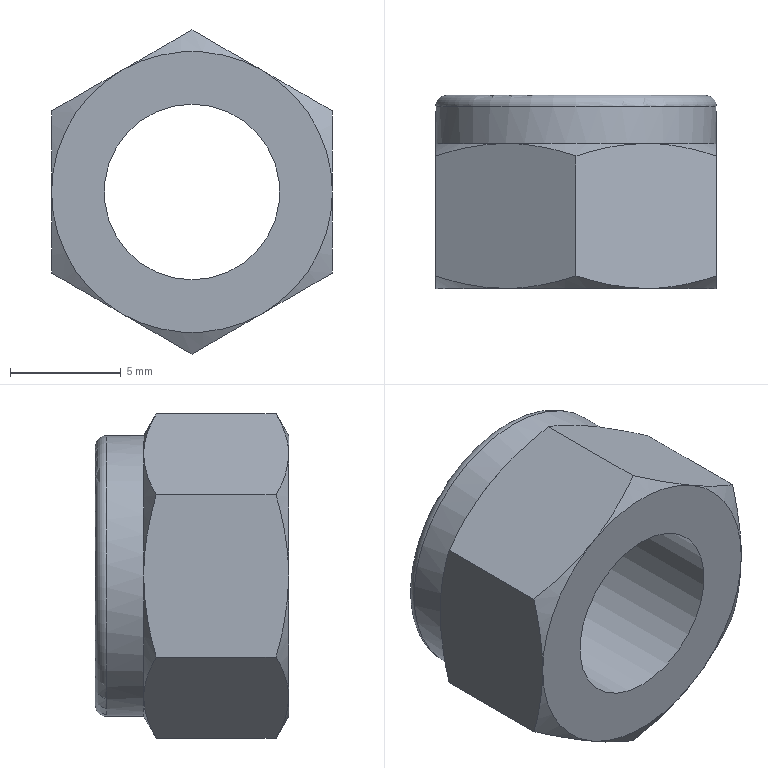Part | NX | features solid 2 | 1 solid | 23 faces | box 12.7 x 8.738 x 14.665 mm | volume 753.009 mm3 | cone 12 | plane 8 | cylinder 2 | torus 1 | commonest cylinder face diameters 7.938 x1 12.7 x1
STEP:
#1=CARTESIAN_POINT('',(0.,5.986,7.332));
#2=VERTEX_POINT('',#1);
#3=CARTESIAN_POINT('',(3.175,6.553,5.499));
#4=VERTEX_POINT('',#3);
#5=CARTESIAN_POINT('',(0.,5.986,7.332));
#6=CARTESIAN_POINT('',(1.039,6.332,6.733));
#7=CARTESIAN_POINT('',(2.093,6.553,6.124));
#8=CARTESIAN_POINT('',(3.175,6.553,5.499));
#9=B_SPLINE_CURVE_WITH_KNOTS('',3,(#5,#6,#7,#8),.UNSPECIFIED.,.F.,.F.,(4,4),(0.000000238,0.00371),.UNSPECIFIED.);
#10=EDGE_CURVE('',#2,#4,#9,.T.);
#11=ORIENTED_EDGE('',*,*,#10,.T.);
#12=CARTESIAN_POINT('',(-3.175,6.553,5.499));
#13=VERTEX_POINT('',#12);
#14=CARTESIAN_POINT('',(0.,6.553,0.));
#15=DIRECTION('',(0.,-1.,0.));
#16=DIRECTION('',(0.,0.,-1.));
#17=AXIS2_PLACEMENT_3D('',#14,#15,#16);
#18=CIRCLE('',#17,6.35);
#19=EDGE_CURVE('',#4,#13,#18,.T.);
#20=ORIENTED_EDGE('',*,*,#19,.T.);
#21=CARTESIAN_POINT('',(-3.175,6.553,5.499));
#22=CARTESIAN_POINT('',(-2.097,6.553,6.122));
#23=CARTESIAN_POINT('',(-1.036,6.331,6.734));
#24=CARTESIAN_POINT('',(0.,5.986,7.332));
#25=B_SPLINE_CURVE_WITH_KNOTS('',3,(#21,#22,#23,#24),.UNSPECIFIED.,.F.,.F.,(4,4),(0.00371,0.007406),.UNSPECIFIED.);
#26=EDGE_CURVE('',#13,#2,#25,.T.);
#27=ORIENTED_EDGE('',*,*,#26,.T.);
#28=EDGE_LOOP('',(#11,#20,#27));
#29=FACE_BOUND('',#28,.T.);
#30=CARTESIAN_POINT('',(0.,6.553,0.));
#31=DIRECTION('',(0.,-1.,0.));
#32=DIRECTION('',(0.,0.,-1.));
#33=AXIS2_PLACEMENT_3D('',#30,#31,#32);
#34=CONICAL_SURFACE('',#33,6.35,1.047);
#35=ADVANCED_FACE('',(#29),#34,.T.);
#36=CARTESIAN_POINT('',(-6.35,5.986,3.666));
#37=VERTEX_POINT('',#36);
#38=CARTESIAN_POINT('',(-6.35,5.986,3.666));
#39=CARTESIAN_POINT('',(-5.311,6.332,4.266));
#40=CARTESIAN_POINT('',(-4.257,6.553,4.875));
#41=CARTESIAN_POINT('',(-3.175,6.553,5.499));
#42=B_SPLINE_CURVE_WITH_KNOTS('',3,(#38,#39,#40,#41),.UNSPECIFIED.,.F.,.F.,(4,4),(0.000000238,0.00371),.UNSPECIFIED.);
#43=EDGE_CURVE('',#37,#13,#42,.T.);
#44=ORIENTED_EDGE('',*,*,#43,.T.);
#45=CARTESIAN_POINT('',(-6.35,6.553,0.));
#46=VERTEX_POINT('',#45);
#47=CARTESIAN_POINT('',(0.,6.553,0.));
#48=DIRECTION('',(0.,-1.,0.));
#49=DIRECTION('',(0.,0.,-1.));
#50=AXIS2_PLACEMENT_3D('',#47,#48,#49);
#51=CIRCLE('',#50,6.35);
#52=EDGE_CURVE('',#13,#46,#51,.T.);
#53=ORIENTED_EDGE('',*,*,#52,.T.);
#54=CARTESIAN_POINT('',(-6.35,6.553,0.));
#55=CARTESIAN_POINT('',(-6.35,6.553,1.241));
#56=CARTESIAN_POINT('',(-6.35,6.328,2.48));
#57=CARTESIAN_POINT('',(-6.35,5.986,3.666));
#58=B_SPLINE_CURVE_WITH_KNOTS('',3,(#54,#55,#56,#57),.UNSPECIFIED.,.F.,.F.,(4,4),(0.01042,0.01413),.UNSPECIFIED.);
#59=EDGE_CURVE('',#46,#37,#58,.T.);
#60=ORIENTED_EDGE('',*,*,#59,.T.);
#61=EDGE_LOOP('',(#44,#53,#60));
#62=FACE_BOUND('',#61,.T.);
#63=CARTESIAN_POINT('',(0.,6.553,0.));
#64=DIRECTION('',(0.,-1.,0.));
#65=DIRECTION('',(0.,0.,-1.));
#66=AXIS2_PLACEMENT_3D('',#63,#64,#65);
#67=CONICAL_SURFACE('',#66,6.35,1.047);
#68=ADVANCED_FACE('',(#62),#67,.T.);
#69=CARTESIAN_POINT('',(-6.35,5.986,-3.666));
#70=VERTEX_POINT('',#69);
#71=CARTESIAN_POINT('',(-6.35,5.986,-3.666));
#72=CARTESIAN_POINT('',(-6.35,6.331,-2.473));
#73=CARTESIAN_POINT('',(-6.35,6.553,-1.24));
#74=CARTESIAN_POINT('',(-6.35,6.553,0.));
#75=B_SPLINE_CURVE_WITH_KNOTS('',3,(#71,#72,#73,#74),.UNSPECIFIED.,.F.,.F.,(4,4),(0.006707,0.01042),.UNSPECIFIED.);
#76=EDGE_CURVE('',#70,#46,#75,.T.);
#77=ORIENTED_EDGE('',*,*,#76,.T.);
#78=CARTESIAN_POINT('',(-3.175,6.553,-5.499));
#79=VERTEX_POINT('',#78);
#80=CARTESIAN_POINT('',(0.,6.553,0.));
#81=DIRECTION('',(0.,-1.,0.));
#82=DIRECTION('',(0.,0.,-1.));
#83=AXIS2_PLACEMENT_3D('',#80,#81,#82);
#84=CIRCLE('',#83,6.35);
#85=EDGE_CURVE('',#46,#79,#84,.T.);
#86=ORIENTED_EDGE('',*,*,#85,.T.);
#87=CARTESIAN_POINT('',(-3.175,6.553,-5.499));
#88=CARTESIAN_POINT('',(-4.253,6.553,-4.877));
#89=CARTESIAN_POINT('',(-5.314,6.331,-4.264));
#90=CARTESIAN_POINT('',(-6.35,5.986,-3.666));
#91=B_SPLINE_CURVE_WITH_KNOTS('',3,(#87,#88,#89,#90),.UNSPECIFIED.,.F.,.F.,(4,4),(0.00371,0.007406),.UNSPECIFIED.);
#92=EDGE_CURVE('',#79,#70,#91,.T.);
#93=ORIENTED_EDGE('',*,*,#92,.T.);
#94=EDGE_LOOP('',(#77,#86,#93));
#95=FACE_BOUND('',#94,.T.);
#96=CARTESIAN_POINT('',(0.,6.553,0.));
#97=DIRECTION('',(0.,-1.,0.));
#98=DIRECTION('',(0.,0.,-1.));
#99=AXIS2_PLACEMENT_3D('',#96,#97,#98);
#100=CONICAL_SURFACE('',#99,6.35,1.047);
#101=ADVANCED_FACE('',(#95),#100,.T.);
#102=CARTESIAN_POINT('',(0.,5.986,-7.332));
#103=VERTEX_POINT('',#102);
#104=CARTESIAN_POINT('',(0.,5.986,-7.332));
#105=CARTESIAN_POINT('',(-1.039,6.332,-6.733));
#106=CARTESIAN_POINT('',(-2.093,6.553,-6.124));
#107=CARTESIAN_POINT('',(-3.175,6.553,-5.499));
#108=B_SPLINE_CURVE_WITH_KNOTS('',3,(#104,#105,#106,#107),.UNSPECIFIED.,.F.,.F.,(4,4),(0.000000238,0.00371),.UNSPECIFIED.);
#109=EDGE_CURVE('',#103,#79,#108,.T.);
#110=ORIENTED_EDGE('',*,*,#109,.T.);
#111=CARTESIAN_POINT('',(3.175,6.553,-5.499));
#112=VERTEX_POINT('',#111);
#113=CARTESIAN_POINT('',(0.,6.553,0.));
#114=DIRECTION('',(0.,-1.,0.));
#115=DIRECTION('',(0.,0.,-1.));
#116=AXIS2_PLACEMENT_3D('',#113,#114,#115);
#117=CIRCLE('',#116,6.35);
#118=EDGE_CURVE('',#79,#112,#117,.T.);
#119=ORIENTED_EDGE('',*,*,#118,.T.);
#120=CARTESIAN_POINT('',(3.175,6.553,-5.499));
#121=CARTESIAN_POINT('',(2.097,6.553,-6.122));
#122=CARTESIAN_POINT('',(1.036,6.331,-6.734));
#123=CARTESIAN_POINT('',(0.,5.986,-7.332));
#124=B_SPLINE_CURVE_WITH_KNOTS('',3,(#120,#121,#122,#123),.UNSPECIFIED.,.F.,.F.,(4,4),(0.00371,0.007406),.UNSPECIFIED.);
#125=EDGE_CURVE('',#112,#103,#124,.T.);
#126=ORIENTED_EDGE('',*,*,#125,.T.);
#127=EDGE_LOOP('',(#110,#119,#126));
#128=FACE_BOUND('',#127,.T.);
#129=CARTESIAN_POINT('',(0.,6.553,0.));
#130=DIRECTION('',(0.,-1.,0.));
#131=DIRECTION('',(0.,0.,-1.));
#132=AXIS2_PLACEMENT_3D('',#129,#130,#131);
#133=CONICAL_SURFACE('',#132,6.35,1.047);
#134=ADVANCED_FACE('',(#128),#133,.T.);
#135=CARTESIAN_POINT('',(6.35,5.986,-3.666));
#136=VERTEX_POINT('',#135);
#137=CARTESIAN_POINT('',(6.35,5.986,-3.666));
#138=CARTESIAN_POINT('',(5.311,6.332,-4.266));
#139=CARTESIAN_POINT('',(4.257,6.553,-4.875));
#140=CARTESIAN_POINT('',(3.175,6.553,-5.499));
#141=B_SPLINE_CURVE_WITH_KNOTS('',3,(#137,#138,#139,#140),.UNSPECIFIED.,.F.,.F.,(4,4),(0.000000238,0.00371),.UNSPECIFIED.);
#142=EDGE_CURVE('',#136,#112,#141,.T.);
#143=ORIENTED_EDGE('',*,*,#142,.T.);
#144=CARTESIAN_POINT('',(6.35,6.553,0.));
#145=VERTEX_POINT('',#144);
#146=CARTESIAN_POINT('',(0.,6.553,0.));
#147=DIRECTION('',(0.,-1.,0.));
#148=DIRECTION('',(0.,0.,-1.));
#149=AXIS2_PLACEMENT_3D('',#146,#147,#148);
#150=CIRCLE('',#149,6.35);
#151=EDGE_CURVE('',#112,#145,#150,.T.);
#152=ORIENTED_EDGE('',*,*,#151,.T.);
#153=CARTESIAN_POINT('',(6.35,5.986,-3.666));
#154=CARTESIAN_POINT('',(6.35,6.331,-2.473));
#155=CARTESIAN_POINT('',(6.35,6.553,-1.24));
#156=CARTESIAN_POINT('',(6.35,6.553,0.));
#157=B_SPLINE_CURVE_WITH_KNOTS('',3,(#153,#154,#155,#156),.UNSPECIFIED.,.F.,.F.,(4,4),(0.006707,0.01042),.UNSPECIFIED.);
#158=EDGE_CURVE('',#145,#136,#157,.F.);
#159=ORIENTED_EDGE('',*,*,#158,.T.);
#160=EDGE_LOOP('',(#143,#152,#159));
#161=FACE_BOUND('',#160,.T.);
#162=CARTESIAN_POINT('',(0.,6.553,0.));
#163=DIRECTION('',(0.,-1.,0.));
#164=DIRECTION('',(0.,0.,-1.));
#165=AXIS2_PLACEMENT_3D('',#162,#163,#164);
#166=CONICAL_SURFACE('',#165,6.35,1.047);
#167=ADVANCED_FACE('',(#161),#166,.T.);
#168=CARTESIAN_POINT('',(-3.175,0.,-5.499));
#169=VERTEX_POINT('',#168);
#170=CARTESIAN_POINT('',(-6.35,0.5672,-3.666));
#171=VERTEX_POINT('',#170);
#172=CARTESIAN_POINT('',(-3.175,0.,-5.499));
#173=CARTESIAN_POINT('',(-4.253,0.,-4.877));
#174=CARTESIAN_POINT('',(-5.314,0.2218,-4.264));
#175=CARTESIAN_POINT('',(-6.35,0.5672,-3.666));
#176=B_SPLINE_CURVE_WITH_KNOTS('',3,(#172,#173,#174,#175),.UNSPECIFIED.,.F.,.F.,(4,4),(0.00371,0.007406),.UNSPECIFIED.);
#177=EDGE_CURVE('',#169,#171,#176,.T.);
#178=ORIENTED_EDGE('',*,*,#177,.F.);
#179=CARTESIAN_POINT('',(-6.35,0.,0.));
#180=VERTEX_POINT('',#179);
#181=CARTESIAN_POINT('',(0.,0.,0.));
#182=DIRECTION('',(0.,-1.,0.));
#183=DIRECTION('',(0.,0.,-1.));
#184=AXIS2_PLACEMENT_3D('',#181,#182,#183);
#185=CIRCLE('',#184,6.35);
#186=EDGE_CURVE('',#180,#169,#185,.T.);
#187=ORIENTED_EDGE('',*,*,#186,.F.);
#188=CARTESIAN_POINT('',(-6.35,0.5672,-3.666));
#189=CARTESIAN_POINT('',(-6.35,0.2226,-2.473));
#190=CARTESIAN_POINT('',(-6.35,0.,-1.24));
#191=CARTESIAN_POINT('',(-6.35,0.,0.));
#192=B_SPLINE_CURVE_WITH_KNOTS('',3,(#188,#189,#190,#191),.UNSPECIFIED.,.F.,.F.,(4,4),(0.006707,0.01042),.UNSPECIFIED.);
#193=EDGE_CURVE('',#171,#180,#192,.T.);
#194=ORIENTED_EDGE('',*,*,#193,.F.);
#195=EDGE_LOOP('',(#178,#187,#194));
#196=FACE_BOUND('',#195,.T.);
#197=CARTESIAN_POINT('',(0.,3.277,0.));
#198=DIRECTION('',(0.,1.,0.));
#199=DIRECTION('',(0.,0.,1.));
#200=AXIS2_PLACEMENT_3D('',#197,#198,#199);
#201=CONICAL_SURFACE('',#200,12.025,1.047);
#202=ADVANCED_FACE('',(#196),#201,.T.);
#203=CARTESIAN_POINT('',(-6.35,0.5672,3.666));
#204=VERTEX_POINT('',#203);
#205=CARTESIAN_POINT('',(-6.35,0.,0.));
#206=CARTESIAN_POINT('',(-6.35,0.,1.241));
#207=CARTESIAN_POINT('',(-6.35,0.2248,2.48));
#208=CARTESIAN_POINT('',(-6.35,0.5672,3.666));
#209=B_SPLINE_CURVE_WITH_KNOTS('',3,(#205,#206,#207,#208),.UNSPECIFIED.,.F.,.F.,(4,4),(0.01042,0.01413),.UNSPECIFIED.);
#210=EDGE_CURVE('',#180,#204,#209,.T.);
#211=ORIENTED_EDGE('',*,*,#210,.F.);
#212=CARTESIAN_POINT('',(-3.175,0.,5.499));
#213=VERTEX_POINT('',#212);
#214=CARTESIAN_POINT('',(0.,0.,0.));
#215=DIRECTION('',(0.,-1.,0.));
#216=DIRECTION('',(0.,0.,-1.));
#217=AXIS2_PLACEMENT_3D('',#214,#215,#216);
#218=CIRCLE('',#217,6.35);
#219=EDGE_CURVE('',#213,#180,#218,.T.);
#220=ORIENTED_EDGE('',*,*,#219,.F.);
#221=CARTESIAN_POINT('',(-6.35,0.5672,3.666));
#222=CARTESIAN_POINT('',(-5.311,0.2209,4.266));
#223=CARTESIAN_POINT('',(-4.257,0.,4.875));
#224=CARTESIAN_POINT('',(-3.175,0.,5.499));
#225=B_SPLINE_CURVE_WITH_KNOTS('',3,(#221,#222,#223,#224),.UNSPECIFIED.,.F.,.F.,(4,4),(0.000000238,0.00371),.UNSPECIFIED.);
#226=EDGE_CURVE('',#204,#213,#225,.T.);
#227=ORIENTED_EDGE('',*,*,#226,.F.);
#228=EDGE_LOOP('',(#211,#220,#227));
#229=FACE_BOUND('',#228,.T.);
#230=CARTESIAN_POINT('',(0.,3.277,0.));
#231=DIRECTION('',(0.,1.,0.));
#232=DIRECTION('',(0.,0.,1.));
#233=AXIS2_PLACEMENT_3D('',#230,#231,#232);
#234=CONICAL_SURFACE('',#233,12.025,1.047);
#235=ADVANCED_FACE('',(#229),#234,.T.);
#236=CARTESIAN_POINT('',(0.,0.5672,-7.332));
#237=VERTEX_POINT('',#236);
#238=CARTESIAN_POINT('',(0.,0.5672,-7.332));
#239=CARTESIAN_POINT('',(-1.039,0.2209,-6.733));
#240=CARTESIAN_POINT('',(-2.093,0.,-6.124));
#241=CARTESIAN_POINT('',(-3.175,0.,-5.499));
#242=B_SPLINE_CURVE_WITH_KNOTS('',3,(#238,#239,#240,#241),.UNSPECIFIED.,.F.,.F.,(4,4),(0.000000238,0.00371),.UNSPECIFIED.);
#243=EDGE_CURVE('',#237,#169,#242,.T.);
#244=ORIENTED_EDGE('',*,*,#243,.F.);
#245=CARTESIAN_POINT('',(3.175,0.,-5.499));
#246=VERTEX_POINT('',#245);
#247=CARTESIAN_POINT('',(3.175,0.,-5.499));
#248=CARTESIAN_POINT('',(2.097,0.,-6.122));
#249=CARTESIAN_POINT('',(1.036,0.2218,-6.734));
#250=CARTESIAN_POINT('',(0.,0.5672,-7.332));
#251=B_SPLINE_CURVE_WITH_KNOTS('',3,(#247,#248,#249,#250),.UNSPECIFIED.,.F.,.F.,(4,4),(0.00371,0.007406),.UNSPECIFIED.);
#252=EDGE_CURVE('',#246,#237,#251,.T.);
#253=ORIENTED_EDGE('',*,*,#252,.F.);
#254=CARTESIAN_POINT('',(0.,0.,0.));
#255=DIRECTION('',(0.,-1.,0.));
#256=DIRECTION('',(0.,0.,-1.));
#257=AXIS2_PLACEMENT_3D('',#254,#255,#256);
#258=CIRCLE('',#257,6.35);
#259=EDGE_CURVE('',#169,#246,#258,.T.);
#260=ORIENTED_EDGE('',*,*,#259,.F.);
#261=EDGE_LOOP('',(#244,#253,#260));
#262=FACE_BOUND('',#261,.T.);
#263=CARTESIAN_POINT('',(0.,3.277,0.));
#264=DIRECTION('',(0.,1.,0.));
#265=DIRECTION('',(0.,0.,1.));
#266=AXIS2_PLACEMENT_3D('',#263,#264,#265);
#267=CONICAL_SURFACE('',#266,12.025,1.047);
#268=ADVANCED_FACE('',(#262),#267,.T.);
#269=CARTESIAN_POINT('',(0.,0.5672,7.332));
#270=VERTEX_POINT('',#269);
#271=CARTESIAN_POINT('',(-3.175,0.,5.499));
#272=CARTESIAN_POINT('',(-2.097,0.,6.122));
#273=CARTESIAN_POINT('',(-1.036,0.2218,6.734));
#274=CARTESIAN_POINT('',(0.,0.5672,7.332));
#275=B_SPLINE_CURVE_WITH_KNOTS('',3,(#271,#272,#273,#274),.UNSPECIFIED.,.F.,.F.,(4,4),(0.00371,0.007406),.UNSPECIFIED.);
#276=EDGE_CURVE('',#213,#270,#275,.T.);
#277=ORIENTED_EDGE('',*,*,#276,.F.);
#278=CARTESIAN_POINT('',(3.175,0.,5.499));
#279=VERTEX_POINT('',#278);
#280=CARTESIAN_POINT('',(0.,0.,0.));
#281=DIRECTION('',(0.,-1.,0.));
#282=DIRECTION('',(0.,0.,-1.));
#283=AXIS2_PLACEMENT_3D('',#280,#281,#282);
#284=CIRCLE('',#283,6.35);
#285=EDGE_CURVE('',#279,#213,#284,.T.);
#286=ORIENTED_EDGE('',*,*,#285,.F.);
#287=CARTESIAN_POINT('',(0.,0.5672,7.332));
#288=CARTESIAN_POINT('',(1.039,0.2209,6.733));
#289=CARTESIAN_POINT('',(2.093,0.,6.124));
#290=CARTESIAN_POINT('',(3.175,0.,5.499));
#291=B_SPLINE_CURVE_WITH_KNOTS('',3,(#287,#288,#289,#290),.UNSPECIFIED.,.F.,.F.,(4,4),(0.000000238,0.00371),.UNSPECIFIED.);
#292=EDGE_CURVE('',#270,#279,#291,.T.);
#293=ORIENTED_EDGE('',*,*,#292,.F.);
#294=EDGE_LOOP('',(#277,#286,#293));
#295=FACE_BOUND('',#294,.T.);
#296=CARTESIAN_POINT('',(0.,3.277,0.));
#297=DIRECTION('',(0.,1.,0.));
#298=DIRECTION('',(0.,0.,1.));
#299=AXIS2_PLACEMENT_3D('',#296,#297,#298);
#300=CONICAL_SURFACE('',#299,12.025,1.047);
#301=ADVANCED_FACE('',(#295),#300,.T.);
#302=CARTESIAN_POINT('',(6.35,0.5672,-3.666));
#303=VERTEX_POINT('',#302);
#304=CARTESIAN_POINT('',(6.35,0.5672,-3.666));
#305=CARTESIAN_POINT('',(5.311,0.2209,-4.266));
#306=CARTESIAN_POINT('',(4.257,0.,-4.875));
#307=CARTESIAN_POINT('',(3.175,0.,-5.499));
#308=B_SPLINE_CURVE_WITH_KNOTS('',3,(#304,#305,#306,#307),.UNSPECIFIED.,.F.,.F.,(4,4),(0.000000238,0.00371),.UNSPECIFIED.);
#309=EDGE_CURVE('',#303,#246,#308,.T.);
#310=ORIENTED_EDGE('',*,*,#309,.F.);
#311=CARTESIAN_POINT('',(6.35,0.,0.));
#312=VERTEX_POINT('',#311);
#313=CARTESIAN_POINT('',(6.35,0.5672,-3.666));
#314=CARTESIAN_POINT('',(6.35,0.2226,-2.473));
#315=CARTESIAN_POINT('',(6.35,0.,-1.24));
#316=CARTESIAN_POINT('',(6.35,0.,0.));
#317=B_SPLINE_CURVE_WITH_KNOTS('',3,(#313,#314,#315,#316),.UNSPECIFIED.,.F.,.F.,(4,4),(0.006707,0.01042),.UNSPECIFIED.);
#318=EDGE_CURVE('',#312,#303,#317,.F.);
#319=ORIENTED_EDGE('',*,*,#318,.F.);
#320=CARTESIAN_POINT('',(0.,0.,0.));
#321=DIRECTION('',(0.,-1.,0.));
#322=DIRECTION('',(0.,0.,-1.));
#323=AXIS2_PLACEMENT_3D('',#320,#321,#322);
#324=CIRCLE('',#323,6.35);
#325=EDGE_CURVE('',#246,#312,#324,.T.);
#326=ORIENTED_EDGE('',*,*,#325,.F.);
#327=EDGE_LOOP('',(#310,#319,#326));
#328=FACE_BOUND('',#327,.T.);
#329=CARTESIAN_POINT('',(0.,3.277,0.));
#330=DIRECTION('',(0.,1.,0.));
#331=DIRECTION('',(0.,0.,1.));
#332=AXIS2_PLACEMENT_3D('',#329,#330,#331);
#333=CONICAL_SURFACE('',#332,12.025,1.047);
#334=ADVANCED_FACE('',(#328),#333,.T.);
#335=CARTESIAN_POINT('',(0.,0.,-3.969));
#336=VERTEX_POINT('',#335);
#337=CARTESIAN_POINT('',(0.,0.,0.));
#338=DIRECTION('',(0.,-1.,0.));
#339=DIRECTION('',(0.,0.,-1.));
#340=AXIS2_PLACEMENT_3D('',#337,#338,#339);
#341=CIRCLE('',#340,3.969);
#342=EDGE_CURVE('',#336,#336,#341,.T.);
#343=ORIENTED_EDGE('',*,*,#342,.F.);
#344=EDGE_LOOP('',(#343));
#345=FACE_BOUND('',#344,.T.);
#346=ORIENTED_EDGE('',*,*,#325,.T.);
#347=CARTESIAN_POINT('',(0.,0.,0.));
#348=DIRECTION('',(0.,-1.,0.));
#349=DIRECTION('',(0.,0.,-1.));
#350=AXIS2_PLACEMENT_3D('',#347,#348,#349);
#351=CIRCLE('',#350,6.35);
#352=EDGE_CURVE('',#312,#279,#351,.T.);
#353=ORIENTED_EDGE('',*,*,#352,.T.);
#354=ORIENTED_EDGE('',*,*,#285,.T.);
#355=ORIENTED_EDGE('',*,*,#219,.T.);
#356=ORIENTED_EDGE('',*,*,#186,.T.);
#357=ORIENTED_EDGE('',*,*,#259,.T.);
#358=EDGE_LOOP('',(#346,#353,#354,#355,#356,#357));
#359=FACE_BOUND('',#358,.T.);
#360=CARTESIAN_POINT('',(6.35,0.,0.));
#361=DIRECTION('',(0.,1.,0.));
#362=DIRECTION('',(0.,0.,1.));
#363=AXIS2_PLACEMENT_3D('',#360,#361,#362);
#364=PLANE('',#363);
#365=ADVANCED_FACE('',(#345,#359),#364,.F.);
#366=CARTESIAN_POINT('',(0.,8.738,-3.969));
#367=VERTEX_POINT('',#366);
#368=CARTESIAN_POINT('',(0.,8.738,0.));
#369=DIRECTION('',(0.,-1.,0.));
#370=DIRECTION('',(0.,0.,-1.));
#371=AXIS2_PLACEMENT_3D('',#368,#369,#370);
#372=CIRCLE('',#371,3.969);
#373=EDGE_CURVE('',#367,#367,#372,.T.);
#374=ORIENTED_EDGE('',*,*,#373,.F.);
#375=EDGE_LOOP('',(#374));
#376=FACE_BOUND('',#375,.T.);
#377=ORIENTED_EDGE('',*,*,#342,.T.);
#378=EDGE_LOOP('',(#377));
#379=FACE_BOUND('',#378,.T.);
#380=CARTESIAN_POINT('',(0.,0.,0.));
#381=DIRECTION('',(0.,-1.,0.));
#382=DIRECTION('',(0.,0.,-1.));
#383=AXIS2_PLACEMENT_3D('',#380,#381,#382);
#384=CYLINDRICAL_SURFACE('',#383,3.969);
#385=ADVANCED_FACE('',(#376,#379),#384,.F.);
#386=CARTESIAN_POINT('',(0.,8.738,-5.842));
#387=VERTEX_POINT('',#386);
#388=CARTESIAN_POINT('',(0.,8.738,0.));
#389=DIRECTION('',(0.,-1.,0.));
#390=DIRECTION('',(0.,0.,-1.));
#391=AXIS2_PLACEMENT_3D('',#388,#389,#390);
#392=CIRCLE('',#391,5.842);
#393=EDGE_CURVE('',#387,#387,#392,.F.);
#394=ORIENTED_EDGE('',*,*,#393,.T.);
#395=EDGE_LOOP('',(#394));
#396=FACE_BOUND('',#395,.T.);
#397=ORIENTED_EDGE('',*,*,#373,.T.);
#398=EDGE_LOOP('',(#397));
#399=FACE_BOUND('',#398,.T.);
#400=CARTESIAN_POINT('',(3.969,8.738,0.));
#401=DIRECTION('',(0.,-1.,0.));
#402=DIRECTION('',(0.,0.,-1.));
#403=AXIS2_PLACEMENT_3D('',#400,#401,#402);
#404=PLANE('',#403);
#405=ADVANCED_FACE('',(#396,#399),#404,.F.);
#406=CARTESIAN_POINT('',(0.,8.23,-6.35));
#407=VERTEX_POINT('',#406);
#408=CARTESIAN_POINT('',(0.,8.23,0.));
#409=DIRECTION('',(0.,-1.,0.));
#410=DIRECTION('',(0.,0.,-1.));
#411=AXIS2_PLACEMENT_3D('',#408,#409,#410);
#412=CIRCLE('',#411,6.35);
#413=EDGE_CURVE('',#407,#407,#412,.T.);
#414=ORIENTED_EDGE('',*,*,#413,.T.);
#415=EDGE_LOOP('',(#414));
#416=FACE_BOUND('',#415,.T.);
#417=ORIENTED_EDGE('',*,*,#151,.F.);
#418=ORIENTED_EDGE('',*,*,#118,.F.);
#419=ORIENTED_EDGE('',*,*,#85,.F.);
#420=ORIENTED_EDGE('',*,*,#52,.F.);
#421=ORIENTED_EDGE('',*,*,#19,.F.);
#422=CARTESIAN_POINT('',(0.,6.553,0.));
#423=DIRECTION('',(0.,-1.,0.));
#424=DIRECTION('',(0.,0.,-1.));
#425=AXIS2_PLACEMENT_3D('',#422,#423,#424);
#426=CIRCLE('',#425,6.35);
#427=EDGE_CURVE('',#145,#4,#426,.T.);
#428=ORIENTED_EDGE('',*,*,#427,.F.);
#429=EDGE_LOOP('',(#417,#418,#419,#420,#421,#428));
#430=FACE_BOUND('',#429,.T.);
#431=CARTESIAN_POINT('',(0.,0.,0.));
#432=DIRECTION('',(0.,-1.,0.));
#433=DIRECTION('',(0.,0.,-1.));
#434=AXIS2_PLACEMENT_3D('',#431,#432,#433);
#435=CYLINDRICAL_SURFACE('',#434,6.35);
#436=ADVANCED_FACE('',(#416,#430),#435,.T.);
#437=CARTESIAN_POINT('',(6.35,5.986,3.666));
#438=VERTEX_POINT('',#437);
#439=CARTESIAN_POINT('',(3.175,6.553,5.499));
#440=CARTESIAN_POINT('',(4.253,6.553,4.877));
#441=CARTESIAN_POINT('',(5.314,6.331,4.264));
#442=CARTESIAN_POINT('',(6.35,5.986,3.666));
#443=B_SPLINE_CURVE_WITH_KNOTS('',3,(#439,#440,#441,#442),.UNSPECIFIED.,.F.,.F.,(4,4),(0.00371,0.007406),.UNSPECIFIED.);
#444=EDGE_CURVE('',#4,#438,#443,.T.);
#445=ORIENTED_EDGE('',*,*,#444,.T.);
#446=CARTESIAN_POINT('',(6.35,6.553,0.));
#447=CARTESIAN_POINT('',(6.35,6.553,1.241));
#448=CARTESIAN_POINT('',(6.35,6.328,2.48));
#449=CARTESIAN_POINT('',(6.35,5.986,3.666));
#450=B_SPLINE_CURVE_WITH_KNOTS('',3,(#446,#447,#448,#449),.UNSPECIFIED.,.F.,.F.,(4,4),(0.01042,0.01413),.UNSPECIFIED.);
#451=EDGE_CURVE('',#438,#145,#450,.F.);
#452=ORIENTED_EDGE('',*,*,#451,.T.);
#453=ORIENTED_EDGE('',*,*,#427,.T.);
#454=EDGE_LOOP('',(#445,#452,#453));
#455=FACE_BOUND('',#454,.T.);
#456=CARTESIAN_POINT('',(0.,6.553,0.));
#457=DIRECTION('',(0.,-1.,0.));
#458=DIRECTION('',(0.,0.,-1.));
#459=AXIS2_PLACEMENT_3D('',#456,#457,#458);
#460=CONICAL_SURFACE('',#459,6.35,1.047);
#461=ADVANCED_FACE('',(#455),#460,.T.);
#462=CARTESIAN_POINT('',(6.35,0.5672,3.666));
#463=VERTEX_POINT('',#462);
#464=CARTESIAN_POINT('',(3.175,0.,5.499));
#465=CARTESIAN_POINT('',(4.253,0.,4.877));
#466=CARTESIAN_POINT('',(5.314,0.2218,4.264));
#467=CARTESIAN_POINT('',(6.35,0.5672,3.666));
#468=B_SPLINE_CURVE_WITH_KNOTS('',3,(#464,#465,#466,#467),.UNSPECIFIED.,.F.,.F.,(4,4),(0.00371,0.007406),.UNSPECIFIED.);
#469=EDGE_CURVE('',#279,#463,#468,.T.);
#470=ORIENTED_EDGE('',*,*,#469,.F.);
#471=ORIENTED_EDGE('',*,*,#352,.F.);
#472=CARTESIAN_POINT('',(6.35,0.,0.));
#473=CARTESIAN_POINT('',(6.35,0.,1.241));
#474=CARTESIAN_POINT('',(6.35,0.2248,2.48));
#475=CARTESIAN_POINT('',(6.35,0.5672,3.666));
#476=B_SPLINE_CURVE_WITH_KNOTS('',3,(#472,#473,#474,#475),.UNSPECIFIED.,.F.,.F.,(4,4),(0.01042,0.01413),.UNSPECIFIED.);
#477=EDGE_CURVE('',#463,#312,#476,.F.);
#478=ORIENTED_EDGE('',*,*,#477,.F.);
#479=EDGE_LOOP('',(#470,#471,#478));
#480=FACE_BOUND('',#479,.T.);
#481=CARTESIAN_POINT('',(0.,3.277,0.));
#482=DIRECTION('',(0.,1.,0.));
#483=DIRECTION('',(0.,0.,1.));
#484=AXIS2_PLACEMENT_3D('',#481,#482,#483);
#485=CONICAL_SURFACE('',#484,12.025,1.047);
#486=ADVANCED_FACE('',(#480),#485,.T.);
#487=CARTESIAN_POINT('',(-6.35,9.611,3.666));
#488=DIRECTION('',(0.,-1.,0.));
#489=VECTOR('',#488,1000.);
#490=LINE('',#487,#489);
#491=EDGE_CURVE('',#37,#204,#490,.T.);
#492=ORIENTED_EDGE('',*,*,#491,.T.);
#493=ORIENTED_EDGE('',*,*,#226,.T.);
#494=ORIENTED_EDGE('',*,*,#276,.T.);
#495=CARTESIAN_POINT('',(0.,9.611,7.332));
#496=DIRECTION('',(0.,-1.,0.));
#497=VECTOR('',#496,1000.);
#498=LINE('',#495,#497);
#499=EDGE_CURVE('',#2,#270,#498,.T.);
#500=ORIENTED_EDGE('',*,*,#499,.F.);
#501=ORIENTED_EDGE('',*,*,#26,.F.);
#502=ORIENTED_EDGE('',*,*,#43,.F.);
#503=EDGE_LOOP('',(#492,#493,#494,#500,#501,#502));
#504=FACE_BOUND('',#503,.T.);
#505=CARTESIAN_POINT('',(0.,9.611,7.332));
#506=DIRECTION('',(-0.5,0.,0.866));
#507=DIRECTION('',(0.866,0.,0.5));
#508=AXIS2_PLACEMENT_3D('',#505,#506,#507);
#509=PLANE('',#508);
#510=ADVANCED_FACE('',(#504),#509,.T.);
#511=CARTESIAN_POINT('',(-6.35,9.611,-3.666));
#512=DIRECTION('',(0.,-1.,0.));
#513=VECTOR('',#512,1000.);
#514=LINE('',#511,#513);
#515=EDGE_CURVE('',#70,#171,#514,.T.);
#516=ORIENTED_EDGE('',*,*,#515,.T.);
#517=ORIENTED_EDGE('',*,*,#193,.T.);
#518=ORIENTED_EDGE('',*,*,#210,.T.);
#519=ORIENTED_EDGE('',*,*,#491,.F.);
#520=ORIENTED_EDGE('',*,*,#59,.F.);
#521=ORIENTED_EDGE('',*,*,#76,.F.);
#522=EDGE_LOOP('',(#516,#517,#518,#519,#520,#521));
#523=FACE_BOUND('',#522,.T.);
#524=CARTESIAN_POINT('',(-6.35,9.611,3.666));
#525=DIRECTION('',(-1.,0.,0.));
#526=DIRECTION('',(0.,0.,1.));
#527=AXIS2_PLACEMENT_3D('',#524,#525,#526);
#528=PLANE('',#527);
#529=ADVANCED_FACE('',(#523),#528,.T.);
#530=CARTESIAN_POINT('',(0.,9.611,-7.332));
#531=DIRECTION('',(0.,-1.,0.));
#532=VECTOR('',#531,1000.);
#533=LINE('',#530,#532);
#534=EDGE_CURVE('',#103,#237,#533,.T.);
#535=ORIENTED_EDGE('',*,*,#534,.T.);
#536=ORIENTED_EDGE('',*,*,#243,.T.);
#537=ORIENTED_EDGE('',*,*,#177,.T.);
#538=ORIENTED_EDGE('',*,*,#515,.F.);
#539=ORIENTED_EDGE('',*,*,#92,.F.);
#540=ORIENTED_EDGE('',*,*,#109,.F.);
#541=EDGE_LOOP('',(#535,#536,#537,#538,#539,#540));
#542=FACE_BOUND('',#541,.T.);
#543=CARTESIAN_POINT('',(-6.35,9.611,-3.666));
#544=DIRECTION('',(-0.5,0.,-0.866));
#545=DIRECTION('',(-0.866,0.,0.5));
#546=AXIS2_PLACEMENT_3D('',#543,#544,#545);
#547=PLANE('',#546);
#548=ADVANCED_FACE('',(#542),#547,.T.);
#549=CARTESIAN_POINT('',(6.35,9.611,-3.666));
#550=DIRECTION('',(0.,-1.,0.));
#551=VECTOR('',#550,1000.);
#552=LINE('',#549,#551);
#553=EDGE_CURVE('',#136,#303,#552,.T.);
#554=ORIENTED_EDGE('',*,*,#553,.T.);
#555=ORIENTED_EDGE('',*,*,#309,.T.);
#556=ORIENTED_EDGE('',*,*,#252,.T.);
#557=ORIENTED_EDGE('',*,*,#534,.F.);
#558=ORIENTED_EDGE('',*,*,#125,.F.);
#559=ORIENTED_EDGE('',*,*,#142,.F.);
#560=EDGE_LOOP('',(#554,#555,#556,#557,#558,#559));
#561=FACE_BOUND('',#560,.T.);
#562=CARTESIAN_POINT('',(0.,9.611,-7.332));
#563=DIRECTION('',(0.5,0.,-0.866));
#564=DIRECTION('',(-0.866,0.,-0.5));
#565=AXIS2_PLACEMENT_3D('',#562,#563,#564);
#566=PLANE('',#565);
#567=ADVANCED_FACE('',(#561),#566,.T.);
#568=ORIENTED_EDGE('',*,*,#499,.T.);
#569=ORIENTED_EDGE('',*,*,#292,.T.);
#570=ORIENTED_EDGE('',*,*,#469,.T.);
#571=CARTESIAN_POINT('',(6.35,9.611,3.666));
#572=DIRECTION('',(0.,-1.,0.));
#573=VECTOR('',#572,1000.);
#574=LINE('',#571,#573);
#575=EDGE_CURVE('',#438,#463,#574,.T.);
#576=ORIENTED_EDGE('',*,*,#575,.F.);
#577=ORIENTED_EDGE('',*,*,#444,.F.);
#578=ORIENTED_EDGE('',*,*,#10,.F.);
#579=EDGE_LOOP('',(#568,#569,#570,#576,#577,#578));
#580=FACE_BOUND('',#579,.T.);
#581=CARTESIAN_POINT('',(6.35,9.611,3.666));
#582=DIRECTION('',(0.5,0.,0.866));
#583=DIRECTION('',(0.866,0.,-0.5));
#584=AXIS2_PLACEMENT_3D('',#581,#582,#583);
#585=PLANE('',#584);
#586=ADVANCED_FACE('',(#580),#585,.T.);
#587=ORIENTED_EDGE('',*,*,#575,.T.);
#588=ORIENTED_EDGE('',*,*,#477,.T.);
#589=ORIENTED_EDGE('',*,*,#318,.T.);
#590=ORIENTED_EDGE('',*,*,#553,.F.);
#591=ORIENTED_EDGE('',*,*,#158,.F.);
#592=ORIENTED_EDGE('',*,*,#451,.F.);
#593=EDGE_LOOP('',(#587,#588,#589,#590,#591,#592));
#594=FACE_BOUND('',#593,.T.);
#595=CARTESIAN_POINT('',(6.35,9.611,-3.666));
#596=DIRECTION('',(1.,0.,0.));
#597=DIRECTION('',(0.,0.,-1.));
#598=AXIS2_PLACEMENT_3D('',#595,#596,#597);
#599=PLANE('',#598);
#600=ADVANCED_FACE('',(#594),#599,.T.);
#601=ORIENTED_EDGE('',*,*,#393,.F.);
#602=EDGE_LOOP('',(#601));
#603=FACE_BOUND('',#602,.T.);
#604=ORIENTED_EDGE('',*,*,#413,.F.);
#605=EDGE_LOOP('',(#604));
#606=FACE_BOUND('',#605,.T.);
#607=CARTESIAN_POINT('',(0.,8.23,0.));
#608=DIRECTION('',(0.,-1.,0.));
#609=DIRECTION('',(0.,0.,-1.));
#610=AXIS2_PLACEMENT_3D('',#607,#608,#609);
#611=TOROIDAL_SURFACE('',#610,5.842,0.508);
#612=ADVANCED_FACE('',(#603,#606),#611,.T.);
#613=CLOSED_SHELL('',(#35,#68,#101,#134,#167,#202,#235,#268,#301,#334,#365,#385,#405,#436,#461,#486,#510,#529,#548,#567,#586,#600,#612));
#614=MANIFOLD_SOLID_BREP('',#613);
#615=(LENGTH_UNIT()NAMED_UNIT(*)SI_UNIT(.MILLI.,.METRE.));
#616=UNCERTAINTY_MEASURE_WITH_UNIT(LENGTH_MEASURE(0.0508),#615,'','');
#617=(NAMED_UNIT(*)PLANE_ANGLE_UNIT()SI_UNIT($,.RADIAN.));
#618=(NAMED_UNIT(*)SI_UNIT($,.STERADIAN.)SOLID_ANGLE_UNIT());
#619=(GEOMETRIC_REPRESENTATION_CONTEXT(3)GLOBAL_UNCERTAINTY_ASSIGNED_CONTEXT((#616))GLOBAL_UNIT_ASSIGNED_CONTEXT((#615,#617,#618))REPRESENTATION_CONTEXT('',''));
#620=ADVANCED_BREP_SHAPE_REPRESENTATION('',(#614),#619);